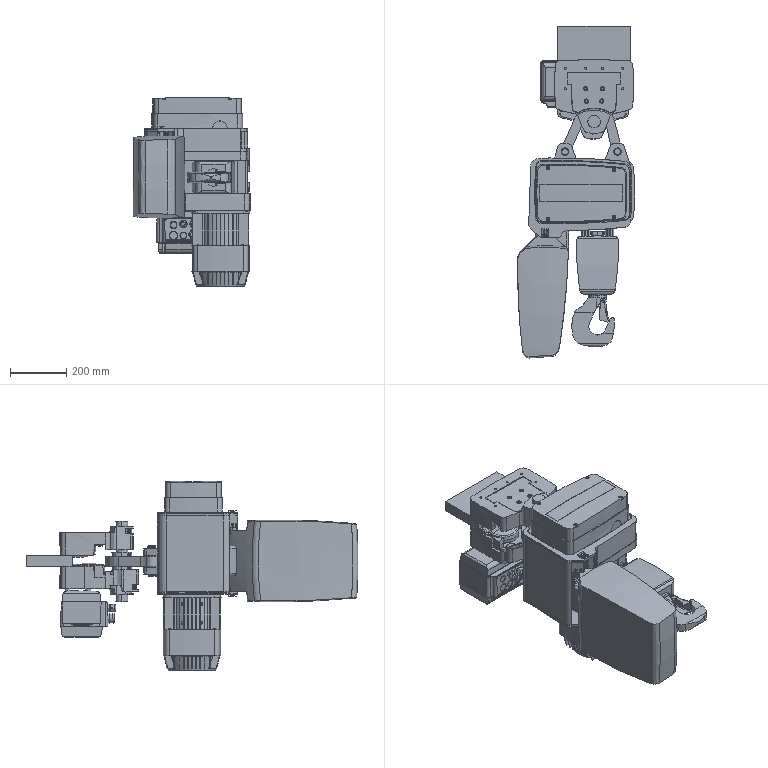Part | SolidWorks | features BaseBody 21, ICE 3, Scale 1 | 22 solids | 3440 faces | volume 83796810 mm3 | plane 1797 | cylinder 1217 | torus 220 | cone 202 | sphere 4 | commonest cylinder face diameters 11 x106 6.6 x58 17.6 x37 7.15 x35 22 x33 172.7 x32